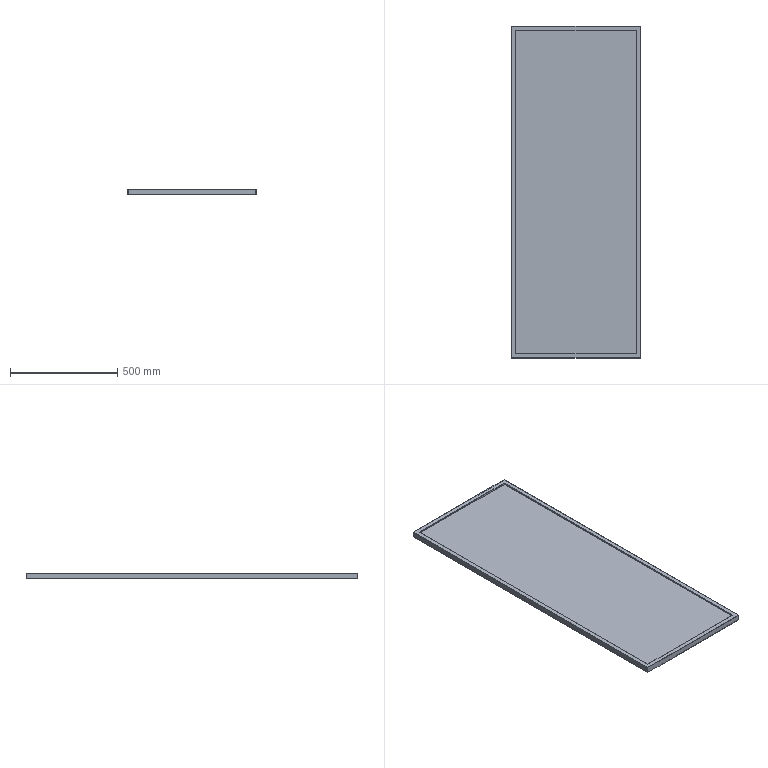Part | SolidWorks | features Extrusion 1, ICE 1, Shell 1 | 1 solid | 16 faces | box 601 x 1551 x 28 mm | volume 2239470 mm3 | plane 16
STEP:
#1=CARTESIAN_POINT('',(0.,1551.,28.));
#2=VERTEX_POINT('',#1);
#3=CARTESIAN_POINT('',(0.,0.,28.));
#4=VERTEX_POINT('',#3);
#5=CARTESIAN_POINT('',(0.,0.,28.));
#6=DIRECTION('',(0.,-1.,0.));
#7=VECTOR('',#6,1000.);
#8=LINE('',#5,#7);
#9=EDGE_CURVE('',#2,#4,#8,.T.);
#10=ORIENTED_EDGE('',*,*,#9,.T.);
#11=CARTESIAN_POINT('',(601.,0.,28.));
#12=VERTEX_POINT('',#11);
#13=CARTESIAN_POINT('',(0.,0.,28.));
#14=DIRECTION('',(1.,0.,0.));
#15=VECTOR('',#14,1000.);
#16=LINE('',#13,#15);
#17=EDGE_CURVE('',#4,#12,#16,.T.);
#18=ORIENTED_EDGE('',*,*,#17,.T.);
#19=CARTESIAN_POINT('',(601.,1551.,28.));
#20=VERTEX_POINT('',#19);
#21=CARTESIAN_POINT('',(601.,0.,28.));
#22=DIRECTION('',(0.,1.,0.));
#23=VECTOR('',#22,1000.);
#24=LINE('',#21,#23);
#25=EDGE_CURVE('',#12,#20,#24,.T.);
#26=ORIENTED_EDGE('',*,*,#25,.T.);
#27=CARTESIAN_POINT('',(0.,1551.,28.));
#28=DIRECTION('',(-1.,0.,0.));
#29=VECTOR('',#28,1000.);
#30=LINE('',#27,#29);
#31=EDGE_CURVE('',#20,#2,#30,.T.);
#32=ORIENTED_EDGE('',*,*,#31,.T.);
#33=EDGE_LOOP('',(#10,#18,#26,#32));
#34=FACE_OUTER_BOUND('',#33,.T.);
#35=CARTESIAN_POINT('',(581.,1531.,28.));
#36=VERTEX_POINT('',#35);
#37=CARTESIAN_POINT('',(20.,1531.,28.));
#38=VERTEX_POINT('',#37);
#39=CARTESIAN_POINT('',(581.,1531.,28.));
#40=DIRECTION('',(-1.,0.,0.));
#41=VECTOR('',#40,1000.);
#42=LINE('',#39,#41);
#43=EDGE_CURVE('',#36,#38,#42,.T.);
#44=ORIENTED_EDGE('',*,*,#43,.F.);
#45=CARTESIAN_POINT('',(581.,20.,28.));
#46=VERTEX_POINT('',#45);
#47=CARTESIAN_POINT('',(581.,20.,28.));
#48=DIRECTION('',(0.,1.,0.));
#49=VECTOR('',#48,1000.);
#50=LINE('',#47,#49);
#51=EDGE_CURVE('',#46,#36,#50,.T.);
#52=ORIENTED_EDGE('',*,*,#51,.F.);
#53=CARTESIAN_POINT('',(20.,20.,28.));
#54=VERTEX_POINT('',#53);
#55=CARTESIAN_POINT('',(20.,20.,28.));
#56=DIRECTION('',(1.,0.,0.));
#57=VECTOR('',#56,1000.);
#58=LINE('',#55,#57);
#59=EDGE_CURVE('',#54,#46,#58,.T.);
#60=ORIENTED_EDGE('',*,*,#59,.F.);
#61=CARTESIAN_POINT('',(20.,1531.,28.));
#62=DIRECTION('',(0.,-1.,0.));
#63=VECTOR('',#62,1000.);
#64=LINE('',#61,#63);
#65=EDGE_CURVE('',#38,#54,#64,.T.);
#66=ORIENTED_EDGE('',*,*,#65,.F.);
#67=EDGE_LOOP('',(#44,#52,#60,#66));
#68=FACE_BOUND('',#67,.T.);
#69=CARTESIAN_POINT('',(0.,1551.,28.));
#70=DIRECTION('',(0.,0.,-1.));
#71=DIRECTION('',(-1.,0.,0.));
#72=AXIS2_PLACEMENT_3D('',#69,#70,#71);
#73=PLANE('',#72);
#74=ADVANCED_FACE('',(#34,#68),#73,.F.);
#75=CARTESIAN_POINT('',(0.,1551.,0.));
#76=VERTEX_POINT('',#75);
#77=CARTESIAN_POINT('',(0.,1551.,28.));
#78=DIRECTION('',(0.,0.,-1.));
#79=VECTOR('',#78,1000.);
#80=LINE('',#77,#79);
#81=EDGE_CURVE('',#2,#76,#80,.T.);
#82=ORIENTED_EDGE('',*,*,#81,.T.);
#83=CARTESIAN_POINT('',(0.,0.,0.));
#84=VERTEX_POINT('',#83);
#85=CARTESIAN_POINT('',(0.,0.,0.));
#86=DIRECTION('',(0.,-1.,0.));
#87=VECTOR('',#86,1000.);
#88=LINE('',#85,#87);
#89=EDGE_CURVE('',#76,#84,#88,.T.);
#90=ORIENTED_EDGE('',*,*,#89,.T.);
#91=CARTESIAN_POINT('',(0.,0.,28.));
#92=DIRECTION('',(0.,0.,-1.));
#93=VECTOR('',#92,1000.);
#94=LINE('',#91,#93);
#95=EDGE_CURVE('',#4,#84,#94,.T.);
#96=ORIENTED_EDGE('',*,*,#95,.F.);
#97=ORIENTED_EDGE('',*,*,#9,.F.);
#98=EDGE_LOOP('',(#82,#90,#96,#97));
#99=FACE_OUTER_BOUND('',#98,.T.);
#100=CARTESIAN_POINT('',(0.,0.,28.));
#101=DIRECTION('',(1.,0.,0.));
#102=DIRECTION('',(0.,0.,-1.));
#103=AXIS2_PLACEMENT_3D('',#100,#101,#102);
#104=PLANE('',#103);
#105=ADVANCED_FACE('',(#99),#104,.F.);
#106=ORIENTED_EDGE('',*,*,#95,.T.);
#107=CARTESIAN_POINT('',(601.,0.,0.));
#108=VERTEX_POINT('',#107);
#109=CARTESIAN_POINT('',(0.,0.,0.));
#110=DIRECTION('',(1.,0.,0.));
#111=VECTOR('',#110,1000.);
#112=LINE('',#109,#111);
#113=EDGE_CURVE('',#84,#108,#112,.T.);
#114=ORIENTED_EDGE('',*,*,#113,.T.);
#115=CARTESIAN_POINT('',(601.,0.,28.));
#116=DIRECTION('',(0.,0.,-1.));
#117=VECTOR('',#116,1000.);
#118=LINE('',#115,#117);
#119=EDGE_CURVE('',#12,#108,#118,.T.);
#120=ORIENTED_EDGE('',*,*,#119,.F.);
#121=ORIENTED_EDGE('',*,*,#17,.F.);
#122=EDGE_LOOP('',(#106,#114,#120,#121));
#123=FACE_OUTER_BOUND('',#122,.T.);
#124=CARTESIAN_POINT('',(0.,0.,28.));
#125=DIRECTION('',(0.,1.,0.));
#126=DIRECTION('',(0.,0.,1.));
#127=AXIS2_PLACEMENT_3D('',#124,#125,#126);
#128=PLANE('',#127);
#129=ADVANCED_FACE('',(#123),#128,.F.);
#130=ORIENTED_EDGE('',*,*,#119,.T.);
#131=CARTESIAN_POINT('',(601.,1551.,0.));
#132=VERTEX_POINT('',#131);
#133=CARTESIAN_POINT('',(601.,0.,0.));
#134=DIRECTION('',(0.,1.,0.));
#135=VECTOR('',#134,1000.);
#136=LINE('',#133,#135);
#137=EDGE_CURVE('',#108,#132,#136,.T.);
#138=ORIENTED_EDGE('',*,*,#137,.T.);
#139=CARTESIAN_POINT('',(601.,1551.,28.));
#140=DIRECTION('',(0.,0.,-1.));
#141=VECTOR('',#140,1000.);
#142=LINE('',#139,#141);
#143=EDGE_CURVE('',#20,#132,#142,.T.);
#144=ORIENTED_EDGE('',*,*,#143,.F.);
#145=ORIENTED_EDGE('',*,*,#25,.F.);
#146=EDGE_LOOP('',(#130,#138,#144,#145));
#147=FACE_OUTER_BOUND('',#146,.T.);
#148=CARTESIAN_POINT('',(601.,0.,28.));
#149=DIRECTION('',(-1.,0.,0.));
#150=DIRECTION('',(0.,0.,1.));
#151=AXIS2_PLACEMENT_3D('',#148,#149,#150);
#152=PLANE('',#151);
#153=ADVANCED_FACE('',(#147),#152,.F.);
#154=ORIENTED_EDGE('',*,*,#143,.T.);
#155=CARTESIAN_POINT('',(0.,1551.,0.));
#156=DIRECTION('',(-1.,0.,0.));
#157=VECTOR('',#156,1000.);
#158=LINE('',#155,#157);
#159=EDGE_CURVE('',#132,#76,#158,.T.);
#160=ORIENTED_EDGE('',*,*,#159,.T.);
#161=ORIENTED_EDGE('',*,*,#81,.F.);
#162=ORIENTED_EDGE('',*,*,#31,.F.);
#163=EDGE_LOOP('',(#154,#160,#161,#162));
#164=FACE_OUTER_BOUND('',#163,.T.);
#165=CARTESIAN_POINT('',(0.,1551.,28.));
#166=DIRECTION('',(0.,-1.,0.));
#167=DIRECTION('',(0.,0.,-1.));
#168=AXIS2_PLACEMENT_3D('',#165,#166,#167);
#169=PLANE('',#168);
#170=ADVANCED_FACE('',(#164),#169,.F.);
#171=ORIENTED_EDGE('',*,*,#89,.F.);
#172=ORIENTED_EDGE('',*,*,#159,.F.);
#173=ORIENTED_EDGE('',*,*,#137,.F.);
#174=ORIENTED_EDGE('',*,*,#113,.F.);
#175=EDGE_LOOP('',(#171,#172,#173,#174));
#176=FACE_OUTER_BOUND('',#175,.T.);
#177=CARTESIAN_POINT('',(0.,1551.,0.));
#178=DIRECTION('',(0.,0.,-1.));
#179=DIRECTION('',(-1.,0.,0.));
#180=AXIS2_PLACEMENT_3D('',#177,#178,#179);
#181=PLANE('',#180);
#182=ADVANCED_FACE('',(#176),#181,.T.);
#183=CARTESIAN_POINT('',(2.,1549.,26.));
#184=VERTEX_POINT('',#183);
#185=CARTESIAN_POINT('',(2.,2.,26.));
#186=VERTEX_POINT('',#185);
#187=CARTESIAN_POINT('',(2.,0.,26.));
#188=DIRECTION('',(0.,-1.,0.));
#189=VECTOR('',#188,1000.);
#190=LINE('',#187,#189);
#191=EDGE_CURVE('',#184,#186,#190,.T.);
#192=ORIENTED_EDGE('',*,*,#191,.F.);
#193=CARTESIAN_POINT('',(599.,1549.,26.));
#194=VERTEX_POINT('',#193);
#195=CARTESIAN_POINT('',(0.,1549.,26.));
#196=DIRECTION('',(-1.,0.,0.));
#197=VECTOR('',#196,1000.);
#198=LINE('',#195,#197);
#199=EDGE_CURVE('',#194,#184,#198,.T.);
#200=ORIENTED_EDGE('',*,*,#199,.F.);
#201=CARTESIAN_POINT('',(599.,2.,26.));
#202=VERTEX_POINT('',#201);
#203=CARTESIAN_POINT('',(599.,0.,26.));
#204=DIRECTION('',(0.,1.,0.));
#205=VECTOR('',#204,1000.);
#206=LINE('',#203,#205);
#207=EDGE_CURVE('',#202,#194,#206,.T.);
#208=ORIENTED_EDGE('',*,*,#207,.F.);
#209=CARTESIAN_POINT('',(0.,2.,26.));
#210=DIRECTION('',(1.,0.,0.));
#211=VECTOR('',#210,1000.);
#212=LINE('',#209,#211);
#213=EDGE_CURVE('',#186,#202,#212,.T.);
#214=ORIENTED_EDGE('',*,*,#213,.F.);
#215=EDGE_LOOP('',(#192,#200,#208,#214));
#216=FACE_OUTER_BOUND('',#215,.T.);
#217=CARTESIAN_POINT('',(581.,20.,26.));
#218=VERTEX_POINT('',#217);
#219=CARTESIAN_POINT('',(581.,1531.,26.));
#220=VERTEX_POINT('',#219);
#221=CARTESIAN_POINT('',(581.,20.,26.));
#222=DIRECTION('',(0.,1.,0.));
#223=VECTOR('',#222,1000.);
#224=LINE('',#221,#223);
#225=EDGE_CURVE('',#218,#220,#224,.T.);
#226=ORIENTED_EDGE('',*,*,#225,.T.);
#227=CARTESIAN_POINT('',(20.,1531.,26.));
#228=VERTEX_POINT('',#227);
#229=CARTESIAN_POINT('',(581.,1531.,26.));
#230=DIRECTION('',(-1.,0.,0.));
#231=VECTOR('',#230,1000.);
#232=LINE('',#229,#231);
#233=EDGE_CURVE('',#220,#228,#232,.T.);
#234=ORIENTED_EDGE('',*,*,#233,.T.);
#235=CARTESIAN_POINT('',(20.,20.,26.));
#236=VERTEX_POINT('',#235);
#237=CARTESIAN_POINT('',(20.,1531.,26.));
#238=DIRECTION('',(0.,-1.,0.));
#239=VECTOR('',#238,1000.);
#240=LINE('',#237,#239);
#241=EDGE_CURVE('',#228,#236,#240,.T.);
#242=ORIENTED_EDGE('',*,*,#241,.T.);
#243=CARTESIAN_POINT('',(20.,20.,26.));
#244=DIRECTION('',(1.,0.,0.));
#245=VECTOR('',#244,1000.);
#246=LINE('',#243,#245);
#247=EDGE_CURVE('',#236,#218,#246,.T.);
#248=ORIENTED_EDGE('',*,*,#247,.T.);
#249=EDGE_LOOP('',(#226,#234,#242,#248));
#250=FACE_BOUND('',#249,.T.);
#251=CARTESIAN_POINT('',(0.,1551.,26.));
#252=DIRECTION('',(0.,0.,1.));
#253=DIRECTION('',(1.,0.,0.));
#254=AXIS2_PLACEMENT_3D('',#251,#252,#253);
#255=PLANE('',#254);
#256=ADVANCED_FACE('',(#216,#250),#255,.F.);
#257=ORIENTED_EDGE('',*,*,#43,.T.);
#258=CARTESIAN_POINT('',(20.,1531.,26.));
#259=DIRECTION('',(0.,0.,1.));
#260=VECTOR('',#259,1000.);
#261=LINE('',#258,#260);
#262=EDGE_CURVE('',#228,#38,#261,.T.);
#263=ORIENTED_EDGE('',*,*,#262,.F.);
#264=ORIENTED_EDGE('',*,*,#233,.F.);
#265=CARTESIAN_POINT('',(581.,1531.,26.));
#266=DIRECTION('',(0.,0.,1.));
#267=VECTOR('',#266,1000.);
#268=LINE('',#265,#267);
#269=EDGE_CURVE('',#220,#36,#268,.T.);
#270=ORIENTED_EDGE('',*,*,#269,.T.);
#271=EDGE_LOOP('',(#257,#263,#264,#270));
#272=FACE_OUTER_BOUND('',#271,.T.);
#273=CARTESIAN_POINT('',(581.,1531.,26.));
#274=DIRECTION('',(0.,1.,0.));
#275=DIRECTION('',(0.,0.,1.));
#276=AXIS2_PLACEMENT_3D('',#273,#274,#275);
#277=PLANE('',#276);
#278=ADVANCED_FACE('',(#272),#277,.F.);
#279=ORIENTED_EDGE('',*,*,#51,.T.);
#280=ORIENTED_EDGE('',*,*,#269,.F.);
#281=ORIENTED_EDGE('',*,*,#225,.F.);
#282=CARTESIAN_POINT('',(581.,20.,26.));
#283=DIRECTION('',(0.,0.,1.));
#284=VECTOR('',#283,1000.);
#285=LINE('',#282,#284);
#286=EDGE_CURVE('',#218,#46,#285,.T.);
#287=ORIENTED_EDGE('',*,*,#286,.T.);
#288=EDGE_LOOP('',(#279,#280,#281,#287));
#289=FACE_OUTER_BOUND('',#288,.T.);
#290=CARTESIAN_POINT('',(581.,20.,26.));
#291=DIRECTION('',(1.,0.,0.));
#292=DIRECTION('',(0.,0.,-1.));
#293=AXIS2_PLACEMENT_3D('',#290,#291,#292);
#294=PLANE('',#293);
#295=ADVANCED_FACE('',(#289),#294,.F.);
#296=ORIENTED_EDGE('',*,*,#59,.T.);
#297=ORIENTED_EDGE('',*,*,#286,.F.);
#298=ORIENTED_EDGE('',*,*,#247,.F.);
#299=CARTESIAN_POINT('',(20.,20.,26.));
#300=DIRECTION('',(0.,0.,1.));
#301=VECTOR('',#300,1000.);
#302=LINE('',#299,#301);
#303=EDGE_CURVE('',#236,#54,#302,.T.);
#304=ORIENTED_EDGE('',*,*,#303,.T.);
#305=EDGE_LOOP('',(#296,#297,#298,#304));
#306=FACE_OUTER_BOUND('',#305,.T.);
#307=CARTESIAN_POINT('',(20.,20.,26.));
#308=DIRECTION('',(0.,-1.,0.));
#309=DIRECTION('',(0.,0.,-1.));
#310=AXIS2_PLACEMENT_3D('',#307,#308,#309);
#311=PLANE('',#310);
#312=ADVANCED_FACE('',(#306),#311,.F.);
#313=ORIENTED_EDGE('',*,*,#65,.T.);
#314=ORIENTED_EDGE('',*,*,#303,.F.);
#315=ORIENTED_EDGE('',*,*,#241,.F.);
#316=ORIENTED_EDGE('',*,*,#262,.T.);
#317=EDGE_LOOP('',(#313,#314,#315,#316));
#318=FACE_OUTER_BOUND('',#317,.T.);
#319=CARTESIAN_POINT('',(20.,1531.,26.));
#320=DIRECTION('',(-1.,0.,0.));
#321=DIRECTION('',(0.,0.,1.));
#322=AXIS2_PLACEMENT_3D('',#319,#320,#321);
#323=PLANE('',#322);
#324=ADVANCED_FACE('',(#318),#323,.F.);
#325=CARTESIAN_POINT('',(2.,1549.,2.));
#326=VERTEX_POINT('',#325);
#327=CARTESIAN_POINT('',(2.,2.,2.));
#328=VERTEX_POINT('',#327);
#329=CARTESIAN_POINT('',(2.,1551.,2.));
#330=DIRECTION('',(0.,-1.,0.));
#331=VECTOR('',#330,1000.);
#332=LINE('',#329,#331);
#333=EDGE_CURVE('',#326,#328,#332,.T.);
#334=ORIENTED_EDGE('',*,*,#333,.T.);
#335=CARTESIAN_POINT('',(599.,2.,2.));
#336=VERTEX_POINT('',#335);
#337=CARTESIAN_POINT('',(0.,2.,2.));
#338=DIRECTION('',(1.,0.,0.));
#339=VECTOR('',#338,1000.);
#340=LINE('',#337,#339);
#341=EDGE_CURVE('',#328,#336,#340,.T.);
#342=ORIENTED_EDGE('',*,*,#341,.T.);
#343=CARTESIAN_POINT('',(599.,1549.,2.));
#344=VERTEX_POINT('',#343);
#345=CARTESIAN_POINT('',(599.,1551.,2.));
#346=DIRECTION('',(0.,1.,0.));
#347=VECTOR('',#346,1000.);
#348=LINE('',#345,#347);
#349=EDGE_CURVE('',#336,#344,#348,.T.);
#350=ORIENTED_EDGE('',*,*,#349,.T.);
#351=CARTESIAN_POINT('',(0.,1549.,2.));
#352=DIRECTION('',(-1.,0.,0.));
#353=VECTOR('',#352,1000.);
#354=LINE('',#351,#353);
#355=EDGE_CURVE('',#344,#326,#354,.T.);
#356=ORIENTED_EDGE('',*,*,#355,.T.);
#357=EDGE_LOOP('',(#334,#342,#350,#356));
#358=FACE_OUTER_BOUND('',#357,.T.);
#359=CARTESIAN_POINT('',(0.,1551.,2.));
#360=DIRECTION('',(0.,0.,-1.));
#361=DIRECTION('',(-1.,0.,0.));
#362=AXIS2_PLACEMENT_3D('',#359,#360,#361);
#363=PLANE('',#362);
#364=ADVANCED_FACE('',(#358),#363,.F.);
#365=CARTESIAN_POINT('',(599.,1549.,28.));
#366=DIRECTION('',(0.,0.,-1.));
#367=VECTOR('',#366,1000.);
#368=LINE('',#365,#367);
#369=EDGE_CURVE('',#194,#344,#368,.T.);
#370=ORIENTED_EDGE('',*,*,#369,.F.);
#371=ORIENTED_EDGE('',*,*,#199,.T.);
#372=CARTESIAN_POINT('',(2.,1549.,28.));
#373=DIRECTION('',(0.,0.,-1.));
#374=VECTOR('',#373,1000.);
#375=LINE('',#372,#374);
#376=EDGE_CURVE('',#184,#326,#375,.T.);
#377=ORIENTED_EDGE('',*,*,#376,.T.);
#378=ORIENTED_EDGE('',*,*,#355,.F.);
#379=EDGE_LOOP('',(#370,#371,#377,#378));
#380=FACE_OUTER_BOUND('',#379,.T.);
#381=CARTESIAN_POINT('',(0.,1549.,28.));
#382=DIRECTION('',(0.,-1.,0.));
#383=DIRECTION('',(0.,0.,-1.));
#384=AXIS2_PLACEMENT_3D('',#381,#382,#383);
#385=PLANE('',#384);
#386=ADVANCED_FACE('',(#380),#385,.T.);
#387=CARTESIAN_POINT('',(599.,2.,28.));
#388=DIRECTION('',(0.,0.,-1.));
#389=VECTOR('',#388,1000.);
#390=LINE('',#387,#389);
#391=EDGE_CURVE('',#202,#336,#390,.T.);
#392=ORIENTED_EDGE('',*,*,#391,.F.);
#393=ORIENTED_EDGE('',*,*,#207,.T.);
#394=ORIENTED_EDGE('',*,*,#369,.T.);
#395=ORIENTED_EDGE('',*,*,#349,.F.);
#396=EDGE_LOOP('',(#392,#393,#394,#395));
#397=FACE_OUTER_BOUND('',#396,.T.);
#398=CARTESIAN_POINT('',(599.,0.,28.));
#399=DIRECTION('',(-1.,0.,0.));
#400=DIRECTION('',(0.,0.,1.));
#401=AXIS2_PLACEMENT_3D('',#398,#399,#400);
#402=PLANE('',#401);
#403=ADVANCED_FACE('',(#397),#402,.T.);
#404=CARTESIAN_POINT('',(2.,2.,28.));
#405=DIRECTION('',(0.,0.,-1.));
#406=VECTOR('',#405,1000.);
#407=LINE('',#404,#406);
#408=EDGE_CURVE('',#186,#328,#407,.T.);
#409=ORIENTED_EDGE('',*,*,#408,.F.);
#410=ORIENTED_EDGE('',*,*,#213,.T.);
#411=ORIENTED_EDGE('',*,*,#391,.T.);
#412=ORIENTED_EDGE('',*,*,#341,.F.);
#413=EDGE_LOOP('',(#409,#410,#411,#412));
#414=FACE_OUTER_BOUND('',#413,.T.);
#415=CARTESIAN_POINT('',(0.,2.,28.));
#416=DIRECTION('',(0.,1.,0.));
#417=DIRECTION('',(0.,0.,1.));
#418=AXIS2_PLACEMENT_3D('',#415,#416,#417);
#419=PLANE('',#418);
#420=ADVANCED_FACE('',(#414),#419,.T.);
#421=ORIENTED_EDGE('',*,*,#376,.F.);
#422=ORIENTED_EDGE('',*,*,#191,.T.);
#423=ORIENTED_EDGE('',*,*,#408,.T.);
#424=ORIENTED_EDGE('',*,*,#333,.F.);
#425=EDGE_LOOP('',(#421,#422,#423,#424));
#426=FACE_OUTER_BOUND('',#425,.T.);
#427=CARTESIAN_POINT('',(2.,0.,28.));
#428=DIRECTION('',(1.,0.,0.));
#429=DIRECTION('',(0.,0.,-1.));
#430=AXIS2_PLACEMENT_3D('',#427,#428,#429);
#431=PLANE('',#430);
#432=ADVANCED_FACE('',(#426),#431,.T.);
#433=CLOSED_SHELL('',(#74,#105,#129,#153,#170,#182,#256,#278,#295,#312,#324,#364,#386,#403,#420,#432));
#434=MANIFOLD_SOLID_BREP('',#433);
#435=CARTESIAN_POINT('',(0.,0.,0.));
#436=DIRECTION('',(0.,0.,1.));
#437=DIRECTION('',(1.,0.,0.));
#438=AXIS2_PLACEMENT_3D('',#435,#436,#437);
#439=(LENGTH_UNIT()NAMED_UNIT(*)SI_UNIT(.MILLI.,.METRE.));
#440=UNCERTAINTY_MEASURE_WITH_UNIT(LENGTH_MEASURE(0.00001),#439,'','');
#441=(NAMED_UNIT(*)PLANE_ANGLE_UNIT()SI_UNIT($,.RADIAN.));
#442=(NAMED_UNIT(*)SI_UNIT($,.STERADIAN.)SOLID_ANGLE_UNIT());
#443=(GEOMETRIC_REPRESENTATION_CONTEXT(3)GLOBAL_UNCERTAINTY_ASSIGNED_CONTEXT((#440))GLOBAL_UNIT_ASSIGNED_CONTEXT((#439,#441,#442))REPRESENTATION_CONTEXT('',''));
#444=ADVANCED_BREP_SHAPE_REPRESENTATION('',(#434,#438),#443);